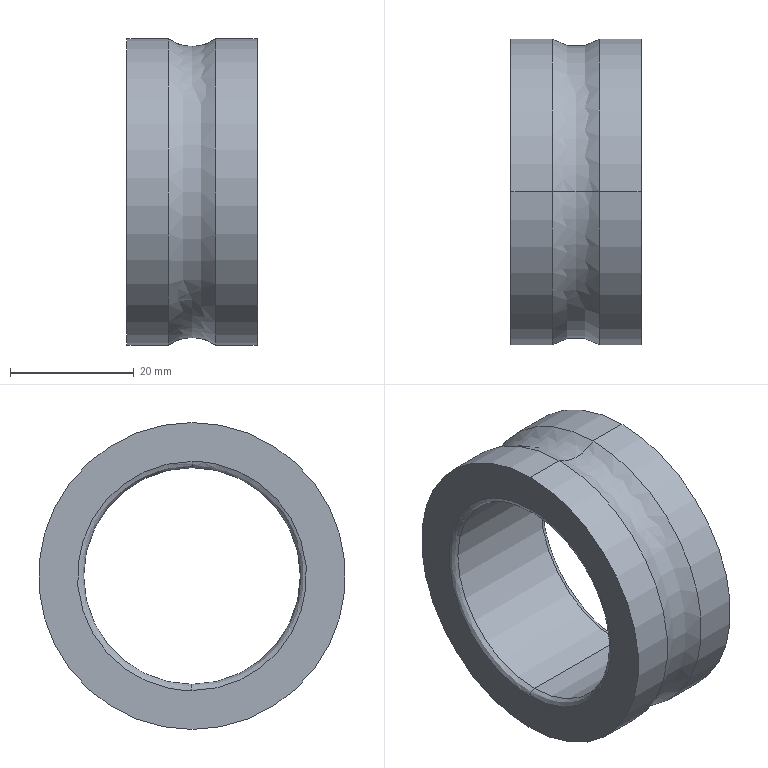Part | STEP file | Inner Ring | 1 solid | 14 faces | box 21 x 49.56 x 49.56 mm | volume 19228 mm3 | spline 6 | cylinder 6 | plane 2 | commonest cylinder face diameters 49.56 x4 35 x2
STEP:
#1=CARTESIAN_POINT('',(1.,0.,17.5));
#2=VERTEX_POINT('',#1);
#3=CARTESIAN_POINT('',(1.,0.,-17.5));
#4=VERTEX_POINT('',#3);
#5=CARTESIAN_POINT('',(1.,0.,0.));
#6=DIRECTION('',(1.,0.,0.));
#7=DIRECTION('',(0.,0.,1.));
#8=AXIS2_PLACEMENT_3D('',#5,#6,#7);
#9=CIRCLE('',#8,17.5);
#10=EDGE_CURVE('',#2,#4,#9,.T.);
#11=ORIENTED_EDGE('',*,*,#10,.T.);
#12=CARTESIAN_POINT('',(0.,0.,-18.5));
#13=VERTEX_POINT('',#12);
#14=CARTESIAN_POINT('',(1.,0.,-18.5));
#15=DIRECTION('',(0.,-1.,0.));
#16=DIRECTION('',(0.,0.,-1.));
#17=AXIS2_PLACEMENT_3D('',#14,#15,#16);
#18=CIRCLE('',#17,1.);
#19=EDGE_CURVE('',#4,#13,#18,.T.);
#20=ORIENTED_EDGE('',*,*,#19,.T.);
#21=CARTESIAN_POINT('',(0.,0.,18.5));
#22=VERTEX_POINT('',#21);
#23=CARTESIAN_POINT('',(0.,0.,-18.5));
#24=CARTESIAN_POINT('',(0.,-37.,-18.5));
#25=CARTESIAN_POINT('',(0.,-37.,18.5));
#26=CARTESIAN_POINT('',(0.,0.,18.5));
#27=(BOUNDED_CURVE()B_SPLINE_CURVE(3,(#23,#24,#25,#26),.UNSPECIFIED.,.F.,.F.)B_SPLINE_CURVE_WITH_KNOTS((4,4),(0.5,1.),.UNSPECIFIED.)CURVE()GEOMETRIC_REPRESENTATION_ITEM()RATIONAL_B_SPLINE_CURVE((1.,0.3333,0.3333,1.))REPRESENTATION_ITEM(''));
#28=EDGE_CURVE('',#13,#22,#27,.T.);
#29=ORIENTED_EDGE('',*,*,#28,.T.);
#30=CARTESIAN_POINT('',(1.,0.,18.5));
#31=DIRECTION('',(0.,1.,0.));
#32=DIRECTION('',(0.,0.,1.));
#33=AXIS2_PLACEMENT_3D('',#30,#31,#32);
#34=CIRCLE('',#33,1.);
#35=EDGE_CURVE('',#2,#22,#34,.T.);
#36=ORIENTED_EDGE('',*,*,#35,.F.);
#37=EDGE_LOOP('',(#11,#20,#29,#36));
#38=FACE_OUTER_BOUND('',#37,.T.);
#39=CARTESIAN_POINT('',(1.,0.,-17.5));
#40=CARTESIAN_POINT('',(1.,-35.,-17.5));
#41=CARTESIAN_POINT('',(1.,-35.,17.5));
#42=CARTESIAN_POINT('',(1.,0.,17.5));
#43=CARTESIAN_POINT('',(0.4142,0.,-17.5));
#44=CARTESIAN_POINT('',(0.4142,-35.,-17.5));
#45=CARTESIAN_POINT('',(0.4142,-35.,17.5));
#46=CARTESIAN_POINT('',(0.4142,0.,17.5));
#47=CARTESIAN_POINT('',(0.,0.,-17.914));
#48=CARTESIAN_POINT('',(0.,-35.828,-17.914));
#49=CARTESIAN_POINT('',(0.,-35.828,17.914));
#50=CARTESIAN_POINT('',(0.,0.,17.914));
#51=CARTESIAN_POINT('',(0.,0.,-18.5));
#52=CARTESIAN_POINT('',(0.,-37.,-18.5));
#53=CARTESIAN_POINT('',(0.,-37.,18.5));
#54=CARTESIAN_POINT('',(0.,0.,18.5));
#55=(BOUNDED_SURFACE()B_SPLINE_SURFACE(3,3,((#39,#40,#41,#42),(#43,#44,#45,#46),(#47,#48,#49,#50),(#51,#52,#53,#54)),.UNSPECIFIED.,.F.,.F.,.F.)B_SPLINE_SURFACE_WITH_KNOTS((4,4),(4,4),(0.,1.),(0.,1.),.UNSPECIFIED.)GEOMETRIC_REPRESENTATION_ITEM()RATIONAL_B_SPLINE_SURFACE(((1.,0.3333,0.3333,1.),(0.8047,0.2682,0.2682,0.8047),(0.8047,0.2682,0.2682,0.8047),(1.,0.3333,0.3333,1.)))REPRESENTATION_ITEM('')SURFACE());
#56=ADVANCED_FACE('',(#38),#55,.T.);
#57=CARTESIAN_POINT('',(20.,0.,-17.5));
#58=VERTEX_POINT('',#57);
#59=CARTESIAN_POINT('',(20.,0.,17.5));
#60=VERTEX_POINT('',#59);
#61=CARTESIAN_POINT('',(20.,0.,0.));
#62=DIRECTION('',(-1.,0.,0.));
#63=DIRECTION('',(0.,0.,1.));
#64=AXIS2_PLACEMENT_3D('',#61,#62,#63);
#65=CIRCLE('',#64,17.5);
#66=EDGE_CURVE('',#58,#60,#65,.T.);
#67=ORIENTED_EDGE('',*,*,#66,.T.);
#68=CARTESIAN_POINT('',(21.,0.,18.5));
#69=VERTEX_POINT('',#68);
#70=CARTESIAN_POINT('',(20.,0.,18.5));
#71=DIRECTION('',(0.,-1.,0.));
#72=DIRECTION('',(0.,0.,1.));
#73=AXIS2_PLACEMENT_3D('',#70,#71,#72);
#74=CIRCLE('',#73,1.);
#75=EDGE_CURVE('',#60,#69,#74,.T.);
#76=ORIENTED_EDGE('',*,*,#75,.T.);
#77=CARTESIAN_POINT('',(21.,0.,-18.5));
#78=VERTEX_POINT('',#77);
#79=CARTESIAN_POINT('',(21.,0.,18.5));
#80=CARTESIAN_POINT('',(21.,-37.,18.5));
#81=CARTESIAN_POINT('',(21.,-37.,-18.5));
#82=CARTESIAN_POINT('',(21.,0.,-18.5));
#83=(BOUNDED_CURVE()B_SPLINE_CURVE(3,(#79,#80,#81,#82),.UNSPECIFIED.,.F.,.F.)B_SPLINE_CURVE_WITH_KNOTS((4,4),(0.5,1.),.UNSPECIFIED.)CURVE()GEOMETRIC_REPRESENTATION_ITEM()RATIONAL_B_SPLINE_CURVE((1.,0.3333,0.3333,1.))REPRESENTATION_ITEM(''));
#84=EDGE_CURVE('',#69,#78,#83,.T.);
#85=ORIENTED_EDGE('',*,*,#84,.T.);
#86=CARTESIAN_POINT('',(20.,0.,-18.5));
#87=DIRECTION('',(0.,1.,0.));
#88=DIRECTION('',(0.,0.,-1.));
#89=AXIS2_PLACEMENT_3D('',#86,#87,#88);
#90=CIRCLE('',#89,1.);
#91=EDGE_CURVE('',#58,#78,#90,.T.);
#92=ORIENTED_EDGE('',*,*,#91,.F.);
#93=EDGE_LOOP('',(#67,#76,#85,#92));
#94=FACE_OUTER_BOUND('',#93,.T.);
#95=CARTESIAN_POINT('',(20.,0.,17.5));
#96=CARTESIAN_POINT('',(20.,-35.,17.5));
#97=CARTESIAN_POINT('',(20.,-35.,-17.5));
#98=CARTESIAN_POINT('',(20.,0.,-17.5));
#99=CARTESIAN_POINT('',(20.586,0.,17.5));
#100=CARTESIAN_POINT('',(20.586,-35.,17.5));
#101=CARTESIAN_POINT('',(20.586,-35.,-17.5));
#102=CARTESIAN_POINT('',(20.586,0.,-17.5));
#103=CARTESIAN_POINT('',(21.,0.,17.914));
#104=CARTESIAN_POINT('',(21.,-35.828,17.914));
#105=CARTESIAN_POINT('',(21.,-35.828,-17.914));
#106=CARTESIAN_POINT('',(21.,0.,-17.914));
#107=CARTESIAN_POINT('',(21.,0.,18.5));
#108=CARTESIAN_POINT('',(21.,-37.,18.5));
#109=CARTESIAN_POINT('',(21.,-37.,-18.5));
#110=CARTESIAN_POINT('',(21.,0.,-18.5));
#111=(BOUNDED_SURFACE()B_SPLINE_SURFACE(3,3,((#95,#96,#97,#98),(#99,#100,#101,#102),(#103,#104,#105,#106),(#107,#108,#109,#110)),.UNSPECIFIED.,.F.,.F.,.F.)B_SPLINE_SURFACE_WITH_KNOTS((4,4),(4,4),(0.,1.),(0.,1.),.UNSPECIFIED.)GEOMETRIC_REPRESENTATION_ITEM()RATIONAL_B_SPLINE_SURFACE(((1.,0.3333,0.3333,1.),(0.8047,0.2682,0.2682,0.8047),(0.8047,0.2682,0.2682,0.8047),(1.,0.3333,0.3333,1.)))REPRESENTATION_ITEM('')SURFACE());
#112=ADVANCED_FACE('',(#94),#111,.T.);
#113=CARTESIAN_POINT('',(14.373,0.,-24.78));
#114=VERTEX_POINT('',#113);
#115=CARTESIAN_POINT('',(14.373,0.,24.78));
#116=VERTEX_POINT('',#115);
#117=CARTESIAN_POINT('',(14.373,0.,0.));
#118=DIRECTION('',(1.,0.,0.));
#119=DIRECTION('',(0.,0.,1.));
#120=AXIS2_PLACEMENT_3D('',#117,#118,#119);
#121=CIRCLE('',#120,24.78);
#122=EDGE_CURVE('',#114,#116,#121,.T.);
#123=ORIENTED_EDGE('',*,*,#122,.F.);
#124=CARTESIAN_POINT('',(6.627,0.,-24.78));
#125=VERTEX_POINT('',#124);
#126=CARTESIAN_POINT('',(10.5,0.,-30.));
#127=DIRECTION('',(0.,-1.,0.));
#128=DIRECTION('',(0.,0.,-1.));
#129=AXIS2_PLACEMENT_3D('',#126,#127,#128);
#130=CIRCLE('',#129,6.5);
#131=EDGE_CURVE('',#114,#125,#130,.T.);
#132=ORIENTED_EDGE('',*,*,#131,.T.);
#133=CARTESIAN_POINT('',(6.627,0.,24.78));
#134=VERTEX_POINT('',#133);
#135=CARTESIAN_POINT('',(6.627,0.,0.));
#136=DIRECTION('',(-1.,0.,0.));
#137=DIRECTION('',(0.,0.,1.));
#138=AXIS2_PLACEMENT_3D('',#135,#136,#137);
#139=CIRCLE('',#138,24.78);
#140=EDGE_CURVE('',#134,#125,#139,.T.);
#141=ORIENTED_EDGE('',*,*,#140,.F.);
#142=CARTESIAN_POINT('',(10.5,0.,30.));
#143=DIRECTION('',(0.,1.,0.));
#144=DIRECTION('',(0.,0.,1.));
#145=AXIS2_PLACEMENT_3D('',#142,#143,#144);
#146=CIRCLE('',#145,6.5);
#147=EDGE_CURVE('',#116,#134,#146,.T.);
#148=ORIENTED_EDGE('',*,*,#147,.F.);
#149=EDGE_LOOP('',(#123,#132,#141,#148));
#150=FACE_OUTER_BOUND('',#149,.T.);
#151=CARTESIAN_POINT('',(14.373,0.,24.78));
#152=CARTESIAN_POINT('',(14.373,49.56,24.78));
#153=CARTESIAN_POINT('',(14.373,49.56,-24.78));
#154=CARTESIAN_POINT('',(14.373,0.,-24.78));
#155=CARTESIAN_POINT('',(11.986,0.,23.009));
#156=CARTESIAN_POINT('',(11.986,46.018,23.009));
#157=CARTESIAN_POINT('',(11.986,46.018,-23.009));
#158=CARTESIAN_POINT('',(11.986,0.,-23.009));
#159=CARTESIAN_POINT('',(9.014,0.,23.009));
#160=CARTESIAN_POINT('',(9.014,46.018,23.009));
#161=CARTESIAN_POINT('',(9.014,46.018,-23.009));
#162=CARTESIAN_POINT('',(9.014,0.,-23.009));
#163=CARTESIAN_POINT('',(6.627,0.,24.78));
#164=CARTESIAN_POINT('',(6.627,49.56,24.78));
#165=CARTESIAN_POINT('',(6.627,49.56,-24.78));
#166=CARTESIAN_POINT('',(6.627,0.,-24.78));
#167=(BOUNDED_SURFACE()B_SPLINE_SURFACE(3,3,((#151,#152,#153,#154),(#155,#156,#157,#158),(#159,#160,#161,#162),(#163,#164,#165,#166)),.UNSPECIFIED.,.F.,.F.,.F.)B_SPLINE_SURFACE_WITH_KNOTS((4,4),(4,4),(0.,1.),(0.,1.),.UNSPECIFIED.)GEOMETRIC_REPRESENTATION_ITEM()RATIONAL_B_SPLINE_SURFACE(((1.,0.3333,0.3333,1.),(0.8687,0.2896,0.2896,0.8687),(0.8687,0.2896,0.2896,0.8687),(1.,0.3333,0.3333,1.)))REPRESENTATION_ITEM('')SURFACE());
#168=ADVANCED_FACE('',(#150),#167,.F.);
#169=ORIENTED_EDGE('',*,*,#66,.F.);
#170=CARTESIAN_POINT('',(-0.4558,0.,-17.5));
#171=DIRECTION('',(-1.,0.,0.));
#172=VECTOR('',#171,1000.);
#173=LINE('',#170,#172);
#174=EDGE_CURVE('',#58,#4,#173,.T.);
#175=ORIENTED_EDGE('',*,*,#174,.T.);
#176=ORIENTED_EDGE('',*,*,#10,.F.);
#177=CARTESIAN_POINT('',(-0.4558,0.,17.5));
#178=DIRECTION('',(-1.,0.,0.));
#179=VECTOR('',#178,1000.);
#180=LINE('',#177,#179);
#181=EDGE_CURVE('',#60,#2,#180,.T.);
#182=ORIENTED_EDGE('',*,*,#181,.F.);
#183=EDGE_LOOP('',(#169,#175,#176,#182));
#184=FACE_OUTER_BOUND('',#183,.T.);
#185=CARTESIAN_POINT('',(-0.4558,0.,0.));
#186=DIRECTION('',(-1.,0.,0.));
#187=DIRECTION('',(0.,0.,1.));
#188=AXIS2_PLACEMENT_3D('',#185,#186,#187);
#189=CYLINDRICAL_SURFACE('',#188,17.5);
#190=ADVANCED_FACE('',(#184),#189,.F.);
#191=ORIENTED_EDGE('',*,*,#140,.T.);
#192=CARTESIAN_POINT('',(0.,0.,-24.78));
#193=VERTEX_POINT('',#192);
#194=CARTESIAN_POINT('',(-0.4558,0.,-24.78));
#195=DIRECTION('',(-1.,0.,0.));
#196=VECTOR('',#195,1000.);
#197=LINE('',#194,#196);
#198=EDGE_CURVE('',#125,#193,#197,.T.);
#199=ORIENTED_EDGE('',*,*,#198,.T.);
#200=CARTESIAN_POINT('',(0.,0.,24.78));
#201=VERTEX_POINT('',#200);
#202=CARTESIAN_POINT('',(0.,0.,0.));
#203=DIRECTION('',(-1.,0.,0.));
#204=DIRECTION('',(0.,0.,1.));
#205=AXIS2_PLACEMENT_3D('',#202,#203,#204);
#206=CIRCLE('',#205,24.78);
#207=EDGE_CURVE('',#201,#193,#206,.T.);
#208=ORIENTED_EDGE('',*,*,#207,.F.);
#209=CARTESIAN_POINT('',(-0.4558,0.,24.78));
#210=DIRECTION('',(-1.,0.,0.));
#211=VECTOR('',#210,1000.);
#212=LINE('',#209,#211);
#213=EDGE_CURVE('',#134,#201,#212,.T.);
#214=ORIENTED_EDGE('',*,*,#213,.F.);
#215=EDGE_LOOP('',(#191,#199,#208,#214));
#216=FACE_OUTER_BOUND('',#215,.T.);
#217=CARTESIAN_POINT('',(-0.4558,0.,0.));
#218=DIRECTION('',(-1.,0.,0.));
#219=DIRECTION('',(0.,0.,1.));
#220=AXIS2_PLACEMENT_3D('',#217,#218,#219);
#221=CYLINDRICAL_SURFACE('',#220,24.78);
#222=ADVANCED_FACE('',(#216),#221,.T.);
#223=CARTESIAN_POINT('',(21.,0.,-24.78));
#224=VERTEX_POINT('',#223);
#225=CARTESIAN_POINT('',(21.,0.,24.78));
#226=VERTEX_POINT('',#225);
#227=CARTESIAN_POINT('',(21.,0.,0.));
#228=DIRECTION('',(1.,0.,0.));
#229=DIRECTION('',(0.,0.,1.));
#230=AXIS2_PLACEMENT_3D('',#227,#228,#229);
#231=CIRCLE('',#230,24.78);
#232=EDGE_CURVE('',#224,#226,#231,.T.);
#233=ORIENTED_EDGE('',*,*,#232,.F.);
#234=CARTESIAN_POINT('',(-0.4558,0.,-24.78));
#235=DIRECTION('',(-1.,0.,0.));
#236=VECTOR('',#235,1000.);
#237=LINE('',#234,#236);
#238=EDGE_CURVE('',#224,#114,#237,.T.);
#239=ORIENTED_EDGE('',*,*,#238,.T.);
#240=ORIENTED_EDGE('',*,*,#122,.T.);
#241=CARTESIAN_POINT('',(-0.4558,0.,24.78));
#242=DIRECTION('',(-1.,0.,0.));
#243=VECTOR('',#242,1000.);
#244=LINE('',#241,#243);
#245=EDGE_CURVE('',#226,#116,#244,.T.);
#246=ORIENTED_EDGE('',*,*,#245,.F.);
#247=EDGE_LOOP('',(#233,#239,#240,#246));
#248=FACE_OUTER_BOUND('',#247,.T.);
#249=CARTESIAN_POINT('',(-0.4558,0.,0.));
#250=DIRECTION('',(-1.,0.,0.));
#251=DIRECTION('',(0.,0.,1.));
#252=AXIS2_PLACEMENT_3D('',#249,#250,#251);
#253=CYLINDRICAL_SURFACE('',#252,24.78);
#254=ADVANCED_FACE('',(#248),#253,.T.);
#255=ORIENTED_EDGE('',*,*,#174,.F.);
#256=CARTESIAN_POINT('',(20.,0.,0.));
#257=DIRECTION('',(-1.,0.,0.));
#258=DIRECTION('',(0.,0.,1.));
#259=AXIS2_PLACEMENT_3D('',#256,#257,#258);
#260=CIRCLE('',#259,17.5);
#261=EDGE_CURVE('',#60,#58,#260,.T.);
#262=ORIENTED_EDGE('',*,*,#261,.F.);
#263=ORIENTED_EDGE('',*,*,#181,.T.);
#264=CARTESIAN_POINT('',(1.,0.,0.));
#265=DIRECTION('',(1.,0.,0.));
#266=DIRECTION('',(0.,0.,1.));
#267=AXIS2_PLACEMENT_3D('',#264,#265,#266);
#268=CIRCLE('',#267,17.5);
#269=EDGE_CURVE('',#4,#2,#268,.T.);
#270=ORIENTED_EDGE('',*,*,#269,.F.);
#271=EDGE_LOOP('',(#255,#262,#263,#270));
#272=FACE_OUTER_BOUND('',#271,.T.);
#273=CARTESIAN_POINT('',(-0.4558,0.,0.));
#274=DIRECTION('',(-1.,0.,0.));
#275=DIRECTION('',(0.,0.,1.));
#276=AXIS2_PLACEMENT_3D('',#273,#274,#275);
#277=CYLINDRICAL_SURFACE('',#276,17.5);
#278=ADVANCED_FACE('',(#272),#277,.F.);
#279=ORIENTED_EDGE('',*,*,#19,.F.);
#280=ORIENTED_EDGE('',*,*,#269,.T.);
#281=ORIENTED_EDGE('',*,*,#35,.T.);
#282=CARTESIAN_POINT('',(0.,0.,18.5));
#283=CARTESIAN_POINT('',(0.,37.,18.5));
#284=CARTESIAN_POINT('',(0.,37.,-18.5));
#285=CARTESIAN_POINT('',(0.,0.,-18.5));
#286=(BOUNDED_CURVE()B_SPLINE_CURVE(3,(#282,#283,#284,#285),.UNSPECIFIED.,.F.,.F.)B_SPLINE_CURVE_WITH_KNOTS((4,4),(0.,0.5),.UNSPECIFIED.)CURVE()GEOMETRIC_REPRESENTATION_ITEM()RATIONAL_B_SPLINE_CURVE((1.,0.3333,0.3333,1.))REPRESENTATION_ITEM(''));
#287=EDGE_CURVE('',#22,#13,#286,.T.);
#288=ORIENTED_EDGE('',*,*,#287,.T.);
#289=EDGE_LOOP('',(#279,#280,#281,#288));
#290=FACE_OUTER_BOUND('',#289,.T.);
#291=CARTESIAN_POINT('',(1.,0.,17.5));
#292=CARTESIAN_POINT('',(1.,35.,17.5));
#293=CARTESIAN_POINT('',(1.,35.,-17.5));
#294=CARTESIAN_POINT('',(1.,0.,-17.5));
#295=CARTESIAN_POINT('',(0.4142,0.,17.5));
#296=CARTESIAN_POINT('',(0.4142,35.,17.5));
#297=CARTESIAN_POINT('',(0.4142,35.,-17.5));
#298=CARTESIAN_POINT('',(0.4142,0.,-17.5));
#299=CARTESIAN_POINT('',(0.,0.,17.914));
#300=CARTESIAN_POINT('',(0.,35.828,17.914));
#301=CARTESIAN_POINT('',(0.,35.828,-17.914));
#302=CARTESIAN_POINT('',(0.,0.,-17.914));
#303=CARTESIAN_POINT('',(0.,0.,18.5));
#304=CARTESIAN_POINT('',(0.,37.,18.5));
#305=CARTESIAN_POINT('',(0.,37.,-18.5));
#306=CARTESIAN_POINT('',(0.,0.,-18.5));
#307=(BOUNDED_SURFACE()B_SPLINE_SURFACE(3,3,((#291,#292,#293,#294),(#295,#296,#297,#298),(#299,#300,#301,#302),(#303,#304,#305,#306)),.UNSPECIFIED.,.F.,.F.,.F.)B_SPLINE_SURFACE_WITH_KNOTS((4,4),(4,4),(0.,1.),(0.,1.),.UNSPECIFIED.)GEOMETRIC_REPRESENTATION_ITEM()RATIONAL_B_SPLINE_SURFACE(((1.,0.3333,0.3333,1.),(0.8047,0.2682,0.2682,0.8047),(0.8047,0.2682,0.2682,0.8047),(1.,0.3333,0.3333,1.)))REPRESENTATION_ITEM('')SURFACE());
#308=ADVANCED_FACE('',(#290),#307,.T.);
#309=ORIENTED_EDGE('',*,*,#75,.F.);
#310=ORIENTED_EDGE('',*,*,#261,.T.);
#311=ORIENTED_EDGE('',*,*,#91,.T.);
#312=CARTESIAN_POINT('',(21.,0.,-18.5));
#313=CARTESIAN_POINT('',(21.,37.,-18.5));
#314=CARTESIAN_POINT('',(21.,37.,18.5));
#315=CARTESIAN_POINT('',(21.,0.,18.5));
#316=(BOUNDED_CURVE()B_SPLINE_CURVE(3,(#312,#313,#314,#315),.UNSPECIFIED.,.F.,.T.)B_SPLINE_CURVE_WITH_KNOTS((4,4),(0.,0.5),.UNSPECIFIED.)CURVE()GEOMETRIC_REPRESENTATION_ITEM()RATIONAL_B_SPLINE_CURVE((1.,0.3333,0.3333,1.))REPRESENTATION_ITEM(''));
#317=EDGE_CURVE('',#78,#69,#316,.T.);
#318=ORIENTED_EDGE('',*,*,#317,.T.);
#319=EDGE_LOOP('',(#309,#310,#311,#318));
#320=FACE_OUTER_BOUND('',#319,.T.);
#321=CARTESIAN_POINT('',(20.,0.,-17.5));
#322=CARTESIAN_POINT('',(20.,35.,-17.5));
#323=CARTESIAN_POINT('',(20.,35.,17.5));
#324=CARTESIAN_POINT('',(20.,0.,17.5));
#325=CARTESIAN_POINT('',(20.586,0.,-17.5));
#326=CARTESIAN_POINT('',(20.586,35.,-17.5));
#327=CARTESIAN_POINT('',(20.586,35.,17.5));
#328=CARTESIAN_POINT('',(20.586,0.,17.5));
#329=CARTESIAN_POINT('',(21.,0.,-17.914));
#330=CARTESIAN_POINT('',(21.,35.828,-17.914));
#331=CARTESIAN_POINT('',(21.,35.828,17.914));
#332=CARTESIAN_POINT('',(21.,0.,17.914));
#333=CARTESIAN_POINT('',(21.,0.,-18.5));
#334=CARTESIAN_POINT('',(21.,37.,-18.5));
#335=CARTESIAN_POINT('',(21.,37.,18.5));
#336=CARTESIAN_POINT('',(21.,0.,18.5));
#337=(BOUNDED_SURFACE()B_SPLINE_SURFACE(3,3,((#321,#322,#323,#324),(#325,#326,#327,#328),(#329,#330,#331,#332),(#333,#334,#335,#336)),.UNSPECIFIED.,.F.,.F.,.F.)B_SPLINE_SURFACE_WITH_KNOTS((4,4),(4,4),(0.,1.),(0.,1.),.UNSPECIFIED.)GEOMETRIC_REPRESENTATION_ITEM()RATIONAL_B_SPLINE_SURFACE(((1.,0.3333,0.3333,1.),(0.8047,0.2682,0.2682,0.8047),(0.8047,0.2682,0.2682,0.8047),(1.,0.3333,0.3333,1.)))REPRESENTATION_ITEM('')SURFACE());
#338=ADVANCED_FACE('',(#320),#337,.T.);
#339=ORIENTED_EDGE('',*,*,#207,.T.);
#340=CARTESIAN_POINT('',(0.,0.,0.));
#341=DIRECTION('',(-1.,0.,0.));
#342=DIRECTION('',(0.,0.,1.));
#343=AXIS2_PLACEMENT_3D('',#340,#341,#342);
#344=CIRCLE('',#343,24.78);
#345=EDGE_CURVE('',#193,#201,#344,.T.);
#346=ORIENTED_EDGE('',*,*,#345,.T.);
#347=EDGE_LOOP('',(#339,#346));
#348=FACE_OUTER_BOUND('',#347,.T.);
#349=ORIENTED_EDGE('',*,*,#287,.F.);
#350=ORIENTED_EDGE('',*,*,#28,.F.);
#351=EDGE_LOOP('',(#349,#350));
#352=FACE_BOUND('',#351,.T.);
#353=CARTESIAN_POINT('',(0.,0.,17.5));
#354=DIRECTION('',(-1.,0.,0.));
#355=DIRECTION('',(0.,0.,1.));
#356=AXIS2_PLACEMENT_3D('',#353,#354,#355);
#357=PLANE('',#356);
#358=ADVANCED_FACE('',(#348,#352),#357,.T.);
#359=CARTESIAN_POINT('',(21.,0.,0.));
#360=DIRECTION('',(1.,0.,0.));
#361=DIRECTION('',(0.,0.,1.));
#362=AXIS2_PLACEMENT_3D('',#359,#360,#361);
#363=CIRCLE('',#362,24.78);
#364=EDGE_CURVE('',#226,#224,#363,.T.);
#365=ORIENTED_EDGE('',*,*,#364,.T.);
#366=ORIENTED_EDGE('',*,*,#232,.T.);
#367=EDGE_LOOP('',(#365,#366));
#368=FACE_OUTER_BOUND('',#367,.T.);
#369=ORIENTED_EDGE('',*,*,#317,.F.);
#370=ORIENTED_EDGE('',*,*,#84,.F.);
#371=EDGE_LOOP('',(#369,#370));
#372=FACE_BOUND('',#371,.T.);
#373=CARTESIAN_POINT('',(21.,0.,24.78));
#374=DIRECTION('',(1.,0.,0.));
#375=DIRECTION('',(0.,0.,-1.));
#376=AXIS2_PLACEMENT_3D('',#373,#374,#375);
#377=PLANE('',#376);
#378=ADVANCED_FACE('',(#368,#372),#377,.T.);
#379=ORIENTED_EDGE('',*,*,#198,.F.);
#380=CARTESIAN_POINT('',(6.627,0.,0.));
#381=DIRECTION('',(-1.,0.,0.));
#382=DIRECTION('',(0.,0.,1.));
#383=AXIS2_PLACEMENT_3D('',#380,#381,#382);
#384=CIRCLE('',#383,24.78);
#385=EDGE_CURVE('',#125,#134,#384,.T.);
#386=ORIENTED_EDGE('',*,*,#385,.T.);
#387=ORIENTED_EDGE('',*,*,#213,.T.);
#388=ORIENTED_EDGE('',*,*,#345,.F.);
#389=EDGE_LOOP('',(#379,#386,#387,#388));
#390=FACE_OUTER_BOUND('',#389,.T.);
#391=CARTESIAN_POINT('',(-0.4558,0.,0.));
#392=DIRECTION('',(-1.,0.,0.));
#393=DIRECTION('',(0.,0.,1.));
#394=AXIS2_PLACEMENT_3D('',#391,#392,#393);
#395=CYLINDRICAL_SURFACE('',#394,24.78);
#396=ADVANCED_FACE('',(#390),#395,.T.);
#397=ORIENTED_EDGE('',*,*,#238,.F.);
#398=ORIENTED_EDGE('',*,*,#364,.F.);
#399=ORIENTED_EDGE('',*,*,#245,.T.);
#400=CARTESIAN_POINT('',(14.373,0.,0.));
#401=DIRECTION('',(1.,0.,0.));
#402=DIRECTION('',(0.,0.,1.));
#403=AXIS2_PLACEMENT_3D('',#400,#401,#402);
#404=CIRCLE('',#403,24.78);
#405=EDGE_CURVE('',#116,#114,#404,.T.);
#406=ORIENTED_EDGE('',*,*,#405,.T.);
#407=EDGE_LOOP('',(#397,#398,#399,#406));
#408=FACE_OUTER_BOUND('',#407,.T.);
#409=CARTESIAN_POINT('',(-0.4558,0.,0.));
#410=DIRECTION('',(-1.,0.,0.));
#411=DIRECTION('',(0.,0.,1.));
#412=AXIS2_PLACEMENT_3D('',#409,#410,#411);
#413=CYLINDRICAL_SURFACE('',#412,24.78);
#414=ADVANCED_FACE('',(#408),#413,.T.);
#415=ORIENTED_EDGE('',*,*,#131,.F.);
#416=ORIENTED_EDGE('',*,*,#405,.F.);
#417=ORIENTED_EDGE('',*,*,#147,.T.);
#418=ORIENTED_EDGE('',*,*,#385,.F.);
#419=EDGE_LOOP('',(#415,#416,#417,#418));
#420=FACE_OUTER_BOUND('',#419,.T.);
#421=CARTESIAN_POINT('',(14.373,0.,-24.78));
#422=CARTESIAN_POINT('',(14.373,-49.56,-24.78));
#423=CARTESIAN_POINT('',(14.373,-49.56,24.78));
#424=CARTESIAN_POINT('',(14.373,0.,24.78));
#425=CARTESIAN_POINT('',(11.986,0.,-23.009));
#426=CARTESIAN_POINT('',(11.986,-46.018,-23.009));
#427=CARTESIAN_POINT('',(11.986,-46.018,23.009));
#428=CARTESIAN_POINT('',(11.986,0.,23.009));
#429=CARTESIAN_POINT('',(9.014,0.,-23.009));
#430=CARTESIAN_POINT('',(9.014,-46.018,-23.009));
#431=CARTESIAN_POINT('',(9.014,-46.018,23.009));
#432=CARTESIAN_POINT('',(9.014,0.,23.009));
#433=CARTESIAN_POINT('',(6.627,0.,-24.78));
#434=CARTESIAN_POINT('',(6.627,-49.56,-24.78));
#435=CARTESIAN_POINT('',(6.627,-49.56,24.78));
#436=CARTESIAN_POINT('',(6.627,0.,24.78));
#437=(BOUNDED_SURFACE()B_SPLINE_SURFACE(3,3,((#421,#422,#423,#424),(#425,#426,#427,#428),(#429,#430,#431,#432),(#433,#434,#435,#436)),.UNSPECIFIED.,.F.,.F.,.F.)B_SPLINE_SURFACE_WITH_KNOTS((4,4),(4,4),(0.,1.),(0.,1.),.UNSPECIFIED.)GEOMETRIC_REPRESENTATION_ITEM()RATIONAL_B_SPLINE_SURFACE(((1.,0.3333,0.3333,1.),(0.8687,0.2896,0.2896,0.8687),(0.8687,0.2896,0.2896,0.8687),(1.,0.3333,0.3333,1.)))REPRESENTATION_ITEM('')SURFACE());
#438=ADVANCED_FACE('',(#420),#437,.F.);
#439=CLOSED_SHELL('',(#56,#112,#168,#190,#222,#254,#278,#308,#338,#358,#378,#396,#414,#438));
#440=MANIFOLD_SOLID_BREP('',#439);
#441=CARTESIAN_POINT('',(0.,0.,0.));
#442=DIRECTION('',(0.,0.,1.));
#443=DIRECTION('',(1.,0.,0.));
#444=AXIS2_PLACEMENT_3D('',#441,#442,#443);
#445=(LENGTH_UNIT()NAMED_UNIT(*)SI_UNIT(.MILLI.,.METRE.));
#446=UNCERTAINTY_MEASURE_WITH_UNIT(LENGTH_MEASURE(0.00001),#445,'','');
#447=(NAMED_UNIT(*)PLANE_ANGLE_UNIT()SI_UNIT($,.RADIAN.));
#448=(NAMED_UNIT(*)SI_UNIT($,.STERADIAN.)SOLID_ANGLE_UNIT());
#449=(GEOMETRIC_REPRESENTATION_CONTEXT(3)GLOBAL_UNCERTAINTY_ASSIGNED_CONTEXT((#446))GLOBAL_UNIT_ASSIGNED_CONTEXT((#445,#447,#448))REPRESENTATION_CONTEXT('',''));
#450=ADVANCED_BREP_SHAPE_REPRESENTATION('',(#440,#444),#449);